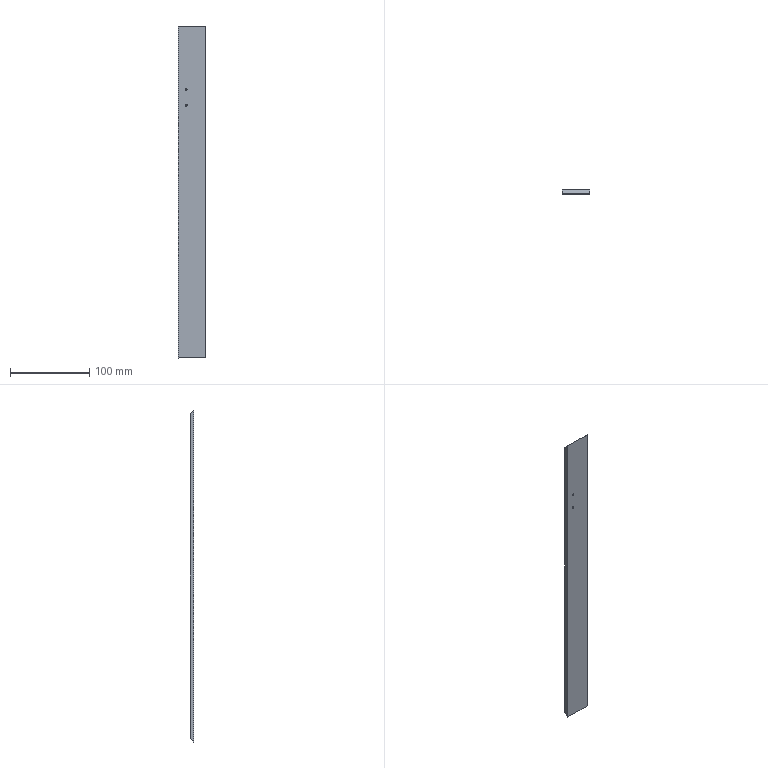Part | STEP file | 09-25 Cover side plate 1 | 1 solid | 10 faces | box 35 x 5 x 420 mm | volume 72576 mm3 | plane 6 | cylinder 4 | commonest cylinder face diameters 2.5 x4
STEP:
#1=CARTESIAN_POINT('',(0.,0.,0.));
#2=DIRECTION('',(0.,0.,1.));
#3=DIRECTION('',(1.,0.,0.));
#4=AXIS2_PLACEMENT_3D('',#1,#2,#3);
#5=CARTESIAN_POINT('',(11.25,5.,-80.));
#6=VERTEX_POINT('',#5);
#7=CARTESIAN_POINT('',(11.25,0.,-80.));
#8=VERTEX_POINT('',#7);
#9=CARTESIAN_POINT('',(11.25,5.,-80.));
#10=DIRECTION('',(0.,-1.,0.));
#11=VECTOR('',#10,1.);
#12=LINE('',#9,#11);
#13=CARTESIAN_POINT('',(10.,5.,-80.));
#14=DIRECTION('',(0.,-1.,0.));
#15=DIRECTION('',(1.,0.,0.));
#16=AXIS2_PLACEMENT_3D('',#13,#14,#15);
#17=CYLINDRICAL_SURFACE('',#16,1.25);
#18=CARTESIAN_POINT('',(6.283,0.));
#19=DIRECTION('',(0.,1.));
#20=VECTOR('',#19,1.);
#21=LINE('',#18,#20);
#22=(GEOMETRIC_REPRESENTATION_CONTEXT(2)PARAMETRIC_REPRESENTATION_CONTEXT()REPRESENTATION_CONTEXT('',''));
#23=DEFINITIONAL_REPRESENTATION('',(#21),#22);
#24=PCURVE('',#17,#23);
#25=CARTESIAN_POINT('',(10.,5.,-80.));
#26=DIRECTION('',(0.,-1.,0.));
#27=DIRECTION('',(1.,0.,0.));
#28=AXIS2_PLACEMENT_3D('',#25,#26,#27);
#29=CYLINDRICAL_SURFACE('',#28,1.25);
#30=CARTESIAN_POINT('',(0.,0.));
#31=DIRECTION('',(0.,1.));
#32=VECTOR('',#31,1.);
#33=LINE('',#30,#32);
#34=(GEOMETRIC_REPRESENTATION_CONTEXT(2)PARAMETRIC_REPRESENTATION_CONTEXT()REPRESENTATION_CONTEXT('',''));
#35=DEFINITIONAL_REPRESENTATION('',(#33),#34);
#36=PCURVE('',#29,#35);
#37=SURFACE_CURVE('',#12,(#24,#36),.PCURVE_S1.);
#38=EDGE_CURVE('',#6,#8,#37,.T.);
#39=ORIENTED_EDGE('',*,*,#38,.T.);
#40=CARTESIAN_POINT('',(8.75,0.,-80.));
#41=VERTEX_POINT('',#40);
#42=CARTESIAN_POINT('',(10.,0.,-80.));
#43=DIRECTION('',(0.,-1.,0.));
#44=DIRECTION('',(1.,0.,0.));
#45=AXIS2_PLACEMENT_3D('',#42,#43,#44);
#46=CIRCLE('',#45,1.25);
#47=CARTESIAN_POINT('',(0.,5.));
#48=DIRECTION('',(1.,0.));
#49=VECTOR('',#48,1.);
#50=LINE('',#47,#49);
#51=(GEOMETRIC_REPRESENTATION_CONTEXT(2)PARAMETRIC_REPRESENTATION_CONTEXT()REPRESENTATION_CONTEXT('',''));
#52=DEFINITIONAL_REPRESENTATION('',(#50),#51);
#53=PCURVE('',#17,#52);
#54=CARTESIAN_POINT('',(0.,0.,-420.));
#55=DIRECTION('',(0.,1.,0.));
#56=DIRECTION('',(0.,0.,1.));
#57=AXIS2_PLACEMENT_3D('',#54,#55,#56);
#58=PLANE('',#57);
#59=CARTESIAN_POINT('',(340.,11.25));
#60=CARTESIAN_POINT('',(342.165,11.25));
#61=CARTESIAN_POINT('',(341.083,9.375));
#62=CARTESIAN_POINT('',(340.,7.5));
#63=CARTESIAN_POINT('',(338.917,9.375));
#64=CARTESIAN_POINT('',(337.835,11.25));
#65=CARTESIAN_POINT('',(340.,11.25));
#66=(BOUNDED_CURVE()B_SPLINE_CURVE(2,(#59,#60,#61,#62,#63,#64,#65),.UNSPECIFIED.,.T.,.F.)B_SPLINE_CURVE_WITH_KNOTS((1,2,2,2,2,1),(-2.094,0.,2.094,4.189,6.283,8.378),.UNSPECIFIED.)CURVE()GEOMETRIC_REPRESENTATION_ITEM()RATIONAL_B_SPLINE_CURVE((1.,0.5,1.,0.5,1.,0.5,1.))REPRESENTATION_ITEM(''));
#67=(GEOMETRIC_REPRESENTATION_CONTEXT(2)PARAMETRIC_REPRESENTATION_CONTEXT()REPRESENTATION_CONTEXT('',''));
#68=DEFINITIONAL_REPRESENTATION('',(#66),#67);
#69=PCURVE('',#58,#68);
#70=SURFACE_CURVE('',#46,(#53,#69),.PCURVE_S1.);
#71=EDGE_CURVE('',#41,#8,#70,.T.);
#72=ORIENTED_EDGE('',*,*,#71,.F.);
#73=CARTESIAN_POINT('',(8.75,5.,-80.));
#74=VERTEX_POINT('',#73);
#75=CARTESIAN_POINT('',(8.75,5.,-80.));
#76=DIRECTION('',(0.,-1.,0.));
#77=VECTOR('',#76,1.);
#78=LINE('',#75,#77);
#79=CARTESIAN_POINT('',(3.142,0.));
#80=DIRECTION('',(0.,1.));
#81=VECTOR('',#80,1.);
#82=LINE('',#79,#81);
#83=(GEOMETRIC_REPRESENTATION_CONTEXT(2)PARAMETRIC_REPRESENTATION_CONTEXT()REPRESENTATION_CONTEXT('',''));
#84=DEFINITIONAL_REPRESENTATION('',(#82),#83);
#85=PCURVE('',#17,#84);
#86=CARTESIAN_POINT('',(3.142,0.));
#87=DIRECTION('',(0.,1.));
#88=VECTOR('',#87,1.);
#89=LINE('',#86,#88);
#90=(GEOMETRIC_REPRESENTATION_CONTEXT(2)PARAMETRIC_REPRESENTATION_CONTEXT()REPRESENTATION_CONTEXT('',''));
#91=DEFINITIONAL_REPRESENTATION('',(#89),#90);
#92=PCURVE('',#29,#91);
#93=SURFACE_CURVE('',#78,(#85,#92),.PCURVE_S1.);
#94=EDGE_CURVE('',#74,#41,#93,.T.);
#95=ORIENTED_EDGE('',*,*,#94,.F.);
#96=CARTESIAN_POINT('',(10.,5.,-80.));
#97=DIRECTION('',(0.,1.,0.));
#98=DIRECTION('',(1.,0.,0.));
#99=AXIS2_PLACEMENT_3D('',#96,#97,#98);
#100=CIRCLE('',#99,1.25);
#101=CARTESIAN_POINT('',(6.283,0.));
#102=DIRECTION('',(-1.,0.));
#103=VECTOR('',#102,1.);
#104=LINE('',#101,#103);
#105=(GEOMETRIC_REPRESENTATION_CONTEXT(2)PARAMETRIC_REPRESENTATION_CONTEXT()REPRESENTATION_CONTEXT('',''));
#106=DEFINITIONAL_REPRESENTATION('',(#104),#105);
#107=PCURVE('',#17,#106);
#108=CARTESIAN_POINT('',(0.,5.,-5.));
#109=DIRECTION('',(0.,-1.,0.));
#110=DIRECTION('',(0.,0.,-1.));
#111=AXIS2_PLACEMENT_3D('',#108,#109,#110);
#112=PLANE('',#111);
#113=CARTESIAN_POINT('',(75.,11.25));
#114=CARTESIAN_POINT('',(77.165,11.25));
#115=CARTESIAN_POINT('',(76.083,9.375));
#116=CARTESIAN_POINT('',(75.,7.5));
#117=CARTESIAN_POINT('',(73.917,9.375));
#118=CARTESIAN_POINT('',(72.835,11.25));
#119=CARTESIAN_POINT('',(75.,11.25));
#120=(BOUNDED_CURVE()B_SPLINE_CURVE(2,(#113,#114,#115,#116,#117,#118,#119),.UNSPECIFIED.,.T.,.F.)B_SPLINE_CURVE_WITH_KNOTS((1,2,2,2,2,1),(-2.094,0.,2.094,4.189,6.283,8.378),.UNSPECIFIED.)CURVE()GEOMETRIC_REPRESENTATION_ITEM()RATIONAL_B_SPLINE_CURVE((1.,0.5,1.,0.5,1.,0.5,1.))REPRESENTATION_ITEM(''));
#121=(GEOMETRIC_REPRESENTATION_CONTEXT(2)PARAMETRIC_REPRESENTATION_CONTEXT()REPRESENTATION_CONTEXT('',''));
#122=DEFINITIONAL_REPRESENTATION('',(#120),#121);
#123=PCURVE('',#112,#122);
#124=SURFACE_CURVE('',#100,(#107,#123),.PCURVE_S1.);
#125=EDGE_CURVE('',#6,#74,#124,.T.);
#126=ORIENTED_EDGE('',*,*,#125,.F.);
#127=EDGE_LOOP('',(#39,#72,#95,#126));
#128=FACE_BOUND('',#127,.F.);
#129=ADVANCED_FACE('',(#128),#17,.F.);
#130=CARTESIAN_POINT('',(11.25,5.,-100.));
#131=VERTEX_POINT('',#130);
#132=CARTESIAN_POINT('',(11.25,0.,-100.));
#133=VERTEX_POINT('',#132);
#134=CARTESIAN_POINT('',(11.25,5.,-100.));
#135=DIRECTION('',(0.,-1.,0.));
#136=VECTOR('',#135,1.);
#137=LINE('',#134,#136);
#138=CARTESIAN_POINT('',(10.,5.,-100.));
#139=DIRECTION('',(0.,-1.,0.));
#140=DIRECTION('',(1.,0.,0.));
#141=AXIS2_PLACEMENT_3D('',#138,#139,#140);
#142=CYLINDRICAL_SURFACE('',#141,1.25);
#143=CARTESIAN_POINT('',(6.283,0.));
#144=DIRECTION('',(0.,1.));
#145=VECTOR('',#144,1.);
#146=LINE('',#143,#145);
#147=(GEOMETRIC_REPRESENTATION_CONTEXT(2)PARAMETRIC_REPRESENTATION_CONTEXT()REPRESENTATION_CONTEXT('',''));
#148=DEFINITIONAL_REPRESENTATION('',(#146),#147);
#149=PCURVE('',#142,#148);
#150=CARTESIAN_POINT('',(10.,5.,-100.));
#151=DIRECTION('',(0.,-1.,0.));
#152=DIRECTION('',(1.,0.,0.));
#153=AXIS2_PLACEMENT_3D('',#150,#151,#152);
#154=CYLINDRICAL_SURFACE('',#153,1.25);
#155=CARTESIAN_POINT('',(0.,0.));
#156=DIRECTION('',(0.,1.));
#157=VECTOR('',#156,1.);
#158=LINE('',#155,#157);
#159=(GEOMETRIC_REPRESENTATION_CONTEXT(2)PARAMETRIC_REPRESENTATION_CONTEXT()REPRESENTATION_CONTEXT('',''));
#160=DEFINITIONAL_REPRESENTATION('',(#158),#159);
#161=PCURVE('',#154,#160);
#162=SURFACE_CURVE('',#137,(#149,#161),.PCURVE_S1.);
#163=EDGE_CURVE('',#131,#133,#162,.T.);
#164=ORIENTED_EDGE('',*,*,#163,.T.);
#165=CARTESIAN_POINT('',(8.75,0.,-100.));
#166=VERTEX_POINT('',#165);
#167=CARTESIAN_POINT('',(10.,0.,-100.));
#168=DIRECTION('',(0.,-1.,0.));
#169=DIRECTION('',(1.,0.,0.));
#170=AXIS2_PLACEMENT_3D('',#167,#168,#169);
#171=CIRCLE('',#170,1.25);
#172=CARTESIAN_POINT('',(0.,5.));
#173=DIRECTION('',(1.,0.));
#174=VECTOR('',#173,1.);
#175=LINE('',#172,#174);
#176=(GEOMETRIC_REPRESENTATION_CONTEXT(2)PARAMETRIC_REPRESENTATION_CONTEXT()REPRESENTATION_CONTEXT('',''));
#177=DEFINITIONAL_REPRESENTATION('',(#175),#176);
#178=PCURVE('',#142,#177);
#179=CARTESIAN_POINT('',(320.,11.25));
#180=CARTESIAN_POINT('',(322.165,11.25));
#181=CARTESIAN_POINT('',(321.083,9.375));
#182=CARTESIAN_POINT('',(320.,7.5));
#183=CARTESIAN_POINT('',(318.917,9.375));
#184=CARTESIAN_POINT('',(317.835,11.25));
#185=CARTESIAN_POINT('',(320.,11.25));
#186=(BOUNDED_CURVE()B_SPLINE_CURVE(2,(#179,#180,#181,#182,#183,#184,#185),.UNSPECIFIED.,.T.,.F.)B_SPLINE_CURVE_WITH_KNOTS((1,2,2,2,2,1),(-2.094,0.,2.094,4.189,6.283,8.378),.UNSPECIFIED.)CURVE()GEOMETRIC_REPRESENTATION_ITEM()RATIONAL_B_SPLINE_CURVE((1.,0.5,1.,0.5,1.,0.5,1.))REPRESENTATION_ITEM(''));
#187=(GEOMETRIC_REPRESENTATION_CONTEXT(2)PARAMETRIC_REPRESENTATION_CONTEXT()REPRESENTATION_CONTEXT('',''));
#188=DEFINITIONAL_REPRESENTATION('',(#186),#187);
#189=PCURVE('',#58,#188);
#190=SURFACE_CURVE('',#171,(#178,#189),.PCURVE_S1.);
#191=EDGE_CURVE('',#166,#133,#190,.T.);
#192=ORIENTED_EDGE('',*,*,#191,.F.);
#193=CARTESIAN_POINT('',(8.75,5.,-100.));
#194=VERTEX_POINT('',#193);
#195=CARTESIAN_POINT('',(8.75,5.,-100.));
#196=DIRECTION('',(0.,-1.,0.));
#197=VECTOR('',#196,1.);
#198=LINE('',#195,#197);
#199=CARTESIAN_POINT('',(3.142,0.));
#200=DIRECTION('',(0.,1.));
#201=VECTOR('',#200,1.);
#202=LINE('',#199,#201);
#203=(GEOMETRIC_REPRESENTATION_CONTEXT(2)PARAMETRIC_REPRESENTATION_CONTEXT()REPRESENTATION_CONTEXT('',''));
#204=DEFINITIONAL_REPRESENTATION('',(#202),#203);
#205=PCURVE('',#142,#204);
#206=CARTESIAN_POINT('',(3.142,0.));
#207=DIRECTION('',(0.,1.));
#208=VECTOR('',#207,1.);
#209=LINE('',#206,#208);
#210=(GEOMETRIC_REPRESENTATION_CONTEXT(2)PARAMETRIC_REPRESENTATION_CONTEXT()REPRESENTATION_CONTEXT('',''));
#211=DEFINITIONAL_REPRESENTATION('',(#209),#210);
#212=PCURVE('',#154,#211);
#213=SURFACE_CURVE('',#198,(#205,#212),.PCURVE_S1.);
#214=EDGE_CURVE('',#194,#166,#213,.T.);
#215=ORIENTED_EDGE('',*,*,#214,.F.);
#216=CARTESIAN_POINT('',(10.,5.,-100.));
#217=DIRECTION('',(0.,1.,0.));
#218=DIRECTION('',(1.,0.,0.));
#219=AXIS2_PLACEMENT_3D('',#216,#217,#218);
#220=CIRCLE('',#219,1.25);
#221=CARTESIAN_POINT('',(6.283,0.));
#222=DIRECTION('',(-1.,0.));
#223=VECTOR('',#222,1.);
#224=LINE('',#221,#223);
#225=(GEOMETRIC_REPRESENTATION_CONTEXT(2)PARAMETRIC_REPRESENTATION_CONTEXT()REPRESENTATION_CONTEXT('',''));
#226=DEFINITIONAL_REPRESENTATION('',(#224),#225);
#227=PCURVE('',#142,#226);
#228=CARTESIAN_POINT('',(95.,11.25));
#229=CARTESIAN_POINT('',(97.165,11.25));
#230=CARTESIAN_POINT('',(96.083,9.375));
#231=CARTESIAN_POINT('',(95.,7.5));
#232=CARTESIAN_POINT('',(93.917,9.375));
#233=CARTESIAN_POINT('',(92.835,11.25));
#234=CARTESIAN_POINT('',(95.,11.25));
#235=(BOUNDED_CURVE()B_SPLINE_CURVE(2,(#228,#229,#230,#231,#232,#233,#234),.UNSPECIFIED.,.T.,.F.)B_SPLINE_CURVE_WITH_KNOTS((1,2,2,2,2,1),(-2.094,0.,2.094,4.189,6.283,8.378),.UNSPECIFIED.)CURVE()GEOMETRIC_REPRESENTATION_ITEM()RATIONAL_B_SPLINE_CURVE((1.,0.5,1.,0.5,1.,0.5,1.))REPRESENTATION_ITEM(''));
#236=(GEOMETRIC_REPRESENTATION_CONTEXT(2)PARAMETRIC_REPRESENTATION_CONTEXT()REPRESENTATION_CONTEXT('',''));
#237=DEFINITIONAL_REPRESENTATION('',(#235),#236);
#238=PCURVE('',#112,#237);
#239=SURFACE_CURVE('',#220,(#227,#238),.PCURVE_S1.);
#240=EDGE_CURVE('',#131,#194,#239,.T.);
#241=ORIENTED_EDGE('',*,*,#240,.F.);
#242=EDGE_LOOP('',(#164,#192,#215,#241));
#243=FACE_BOUND('',#242,.F.);
#244=ADVANCED_FACE('',(#243),#142,.F.);
#245=CARTESIAN_POINT('',(10.,0.,-80.));
#246=DIRECTION('',(0.,-1.,0.));
#247=DIRECTION('',(1.,0.,0.));
#248=AXIS2_PLACEMENT_3D('',#245,#246,#247);
#249=CIRCLE('',#248,1.25);
#250=CARTESIAN_POINT('',(0.,5.));
#251=DIRECTION('',(1.,0.));
#252=VECTOR('',#251,1.);
#253=LINE('',#250,#252);
#254=(GEOMETRIC_REPRESENTATION_CONTEXT(2)PARAMETRIC_REPRESENTATION_CONTEXT()REPRESENTATION_CONTEXT('',''));
#255=DEFINITIONAL_REPRESENTATION('',(#253),#254);
#256=PCURVE('',#29,#255);
#257=CARTESIAN_POINT('',(340.,11.25));
#258=CARTESIAN_POINT('',(342.165,11.25));
#259=CARTESIAN_POINT('',(341.083,9.375));
#260=CARTESIAN_POINT('',(340.,7.5));
#261=CARTESIAN_POINT('',(338.917,9.375));
#262=CARTESIAN_POINT('',(337.835,11.25));
#263=CARTESIAN_POINT('',(340.,11.25));
#264=(BOUNDED_CURVE()B_SPLINE_CURVE(2,(#257,#258,#259,#260,#261,#262,#263),.UNSPECIFIED.,.T.,.F.)B_SPLINE_CURVE_WITH_KNOTS((1,2,2,2,2,1),(-2.094,0.,2.094,4.189,6.283,8.378),.UNSPECIFIED.)CURVE()GEOMETRIC_REPRESENTATION_ITEM()RATIONAL_B_SPLINE_CURVE((1.,0.5,1.,0.5,1.,0.5,1.))REPRESENTATION_ITEM(''));
#265=(GEOMETRIC_REPRESENTATION_CONTEXT(2)PARAMETRIC_REPRESENTATION_CONTEXT()REPRESENTATION_CONTEXT('',''));
#266=DEFINITIONAL_REPRESENTATION('',(#264),#265);
#267=PCURVE('',#58,#266);
#268=SURFACE_CURVE('',#249,(#256,#267),.PCURVE_S1.);
#269=EDGE_CURVE('',#8,#41,#268,.T.);
#270=ORIENTED_EDGE('',*,*,#269,.F.);
#271=ORIENTED_EDGE('',*,*,#38,.F.);
#272=CARTESIAN_POINT('',(10.,5.,-80.));
#273=DIRECTION('',(0.,1.,0.));
#274=DIRECTION('',(1.,0.,0.));
#275=AXIS2_PLACEMENT_3D('',#272,#273,#274);
#276=CIRCLE('',#275,1.25);
#277=CARTESIAN_POINT('',(6.283,0.));
#278=DIRECTION('',(-1.,0.));
#279=VECTOR('',#278,1.);
#280=LINE('',#277,#279);
#281=(GEOMETRIC_REPRESENTATION_CONTEXT(2)PARAMETRIC_REPRESENTATION_CONTEXT()REPRESENTATION_CONTEXT('',''));
#282=DEFINITIONAL_REPRESENTATION('',(#280),#281);
#283=PCURVE('',#29,#282);
#284=CARTESIAN_POINT('',(75.,11.25));
#285=CARTESIAN_POINT('',(77.165,11.25));
#286=CARTESIAN_POINT('',(76.083,9.375));
#287=CARTESIAN_POINT('',(75.,7.5));
#288=CARTESIAN_POINT('',(73.917,9.375));
#289=CARTESIAN_POINT('',(72.835,11.25));
#290=CARTESIAN_POINT('',(75.,11.25));
#291=(BOUNDED_CURVE()B_SPLINE_CURVE(2,(#284,#285,#286,#287,#288,#289,#290),.UNSPECIFIED.,.T.,.F.)B_SPLINE_CURVE_WITH_KNOTS((1,2,2,2,2,1),(-2.094,0.,2.094,4.189,6.283,8.378),.UNSPECIFIED.)CURVE()GEOMETRIC_REPRESENTATION_ITEM()RATIONAL_B_SPLINE_CURVE((1.,0.5,1.,0.5,1.,0.5,1.))REPRESENTATION_ITEM(''));
#292=(GEOMETRIC_REPRESENTATION_CONTEXT(2)PARAMETRIC_REPRESENTATION_CONTEXT()REPRESENTATION_CONTEXT('',''));
#293=DEFINITIONAL_REPRESENTATION('',(#291),#292);
#294=PCURVE('',#112,#293);
#295=SURFACE_CURVE('',#276,(#283,#294),.PCURVE_S1.);
#296=EDGE_CURVE('',#74,#6,#295,.T.);
#297=ORIENTED_EDGE('',*,*,#296,.F.);
#298=ORIENTED_EDGE('',*,*,#94,.T.);
#299=EDGE_LOOP('',(#270,#271,#297,#298));
#300=FACE_BOUND('',#299,.F.);
#301=ADVANCED_FACE('',(#300),#29,.F.);
#302=CARTESIAN_POINT('',(10.,0.,-100.));
#303=DIRECTION('',(0.,-1.,0.));
#304=DIRECTION('',(1.,0.,0.));
#305=AXIS2_PLACEMENT_3D('',#302,#303,#304);
#306=CIRCLE('',#305,1.25);
#307=CARTESIAN_POINT('',(320.,11.25));
#308=CARTESIAN_POINT('',(322.165,11.25));
#309=CARTESIAN_POINT('',(321.083,9.375));
#310=CARTESIAN_POINT('',(320.,7.5));
#311=CARTESIAN_POINT('',(318.917,9.375));
#312=CARTESIAN_POINT('',(317.835,11.25));
#313=CARTESIAN_POINT('',(320.,11.25));
#314=(BOUNDED_CURVE()B_SPLINE_CURVE(2,(#307,#308,#309,#310,#311,#312,#313),.UNSPECIFIED.,.T.,.F.)B_SPLINE_CURVE_WITH_KNOTS((1,2,2,2,2,1),(-2.094,0.,2.094,4.189,6.283,8.378),.UNSPECIFIED.)CURVE()GEOMETRIC_REPRESENTATION_ITEM()RATIONAL_B_SPLINE_CURVE((1.,0.5,1.,0.5,1.,0.5,1.))REPRESENTATION_ITEM(''));
#315=(GEOMETRIC_REPRESENTATION_CONTEXT(2)PARAMETRIC_REPRESENTATION_CONTEXT()REPRESENTATION_CONTEXT('',''));
#316=DEFINITIONAL_REPRESENTATION('',(#314),#315);
#317=PCURVE('',#58,#316);
#318=CARTESIAN_POINT('',(0.,5.));
#319=DIRECTION('',(1.,0.));
#320=VECTOR('',#319,1.);
#321=LINE('',#318,#320);
#322=(GEOMETRIC_REPRESENTATION_CONTEXT(2)PARAMETRIC_REPRESENTATION_CONTEXT()REPRESENTATION_CONTEXT('',''));
#323=DEFINITIONAL_REPRESENTATION('',(#321),#322);
#324=PCURVE('',#154,#323);
#325=SURFACE_CURVE('',#306,(#317,#324),.PCURVE_S1.);
#326=EDGE_CURVE('',#133,#166,#325,.T.);
#327=ORIENTED_EDGE('',*,*,#326,.F.);
#328=ORIENTED_EDGE('',*,*,#191,.F.);
#329=EDGE_LOOP('',(#327,#328));
#330=FACE_BOUND('',#329,.T.);
#331=ORIENTED_EDGE('',*,*,#269,.F.);
#332=ORIENTED_EDGE('',*,*,#71,.F.);
#333=EDGE_LOOP('',(#331,#332));
#334=FACE_BOUND('',#333,.T.);
#335=CARTESIAN_POINT('',(35.,0.,-420.));
#336=VERTEX_POINT('',#335);
#337=CARTESIAN_POINT('',(0.,0.,-420.));
#338=VERTEX_POINT('',#337);
#339=CARTESIAN_POINT('',(17.5,0.,-420.));
#340=DIRECTION('',(-1.,0.,0.));
#341=VECTOR('',#340,1.);
#342=LINE('',#339,#341);
#343=CARTESIAN_POINT('',(0.,17.5));
#344=DIRECTION('',(0.,-1.));
#345=VECTOR('',#344,1.);
#346=LINE('',#343,#345);
#347=(GEOMETRIC_REPRESENTATION_CONTEXT(2)PARAMETRIC_REPRESENTATION_CONTEXT()REPRESENTATION_CONTEXT('',''));
#348=DEFINITIONAL_REPRESENTATION('',(#346),#347);
#349=PCURVE('',#58,#348);
#350=CARTESIAN_POINT('',(0.,5.,-415.));
#351=DIRECTION('',(0.,-0.7071,0.7071));
#352=DIRECTION('',(0.,-0.7071,-0.7071));
#353=AXIS2_PLACEMENT_3D('',#350,#351,#352);
#354=PLANE('',#353);
#355=CARTESIAN_POINT('',(7.071,17.5));
#356=DIRECTION('',(0.,-1.));
#357=VECTOR('',#356,1.);
#358=LINE('',#355,#357);
#359=(GEOMETRIC_REPRESENTATION_CONTEXT(2)PARAMETRIC_REPRESENTATION_CONTEXT()REPRESENTATION_CONTEXT('',''));
#360=DEFINITIONAL_REPRESENTATION('',(#358),#359);
#361=PCURVE('',#354,#360);
#362=SURFACE_CURVE('',#342,(#349,#361),.PCURVE_S1.);
#363=EDGE_CURVE('',#336,#338,#362,.T.);
#364=ORIENTED_EDGE('',*,*,#363,.F.);
#365=CARTESIAN_POINT('',(35.,0.,-0.000000052));
#366=VERTEX_POINT('',#365);
#367=CARTESIAN_POINT('',(35.,0.,-210.));
#368=DIRECTION('',(0.,0.,-1.));
#369=VECTOR('',#368,1.);
#370=LINE('',#367,#369);
#371=CARTESIAN_POINT('',(210.,35.));
#372=DIRECTION('',(-1.,0.));
#373=VECTOR('',#372,1.);
#374=LINE('',#371,#373);
#375=(GEOMETRIC_REPRESENTATION_CONTEXT(2)PARAMETRIC_REPRESENTATION_CONTEXT()REPRESENTATION_CONTEXT('',''));
#376=DEFINITIONAL_REPRESENTATION('',(#374),#375);
#377=PCURVE('',#58,#376);
#378=CARTESIAN_POINT('',(35.,0.,2.52));
#379=DIRECTION('',(1.,0.,0.));
#380=DIRECTION('',(0.,0.,-1.));
#381=AXIS2_PLACEMENT_3D('',#378,#379,#380);
#382=PLANE('',#381);
#383=CARTESIAN_POINT('',(212.52,0.));
#384=DIRECTION('',(1.,0.));
#385=VECTOR('',#384,1.);
#386=LINE('',#383,#385);
#387=(GEOMETRIC_REPRESENTATION_CONTEXT(2)PARAMETRIC_REPRESENTATION_CONTEXT()REPRESENTATION_CONTEXT('',''));
#388=DEFINITIONAL_REPRESENTATION('',(#386),#387);
#389=PCURVE('',#382,#388);
#390=SURFACE_CURVE('',#370,(#377,#389),.PCURVE_S1.);
#391=EDGE_CURVE('',#366,#336,#390,.T.);
#392=ORIENTED_EDGE('',*,*,#391,.F.);
#393=CARTESIAN_POINT('',(0.,0.,0.));
#394=VERTEX_POINT('',#393);
#395=CARTESIAN_POINT('',(17.5,0.,0.));
#396=DIRECTION('',(1.,0.,0.));
#397=VECTOR('',#396,1.);
#398=LINE('',#395,#397);
#399=CARTESIAN_POINT('',(420.,17.5));
#400=DIRECTION('',(0.,1.));
#401=VECTOR('',#400,1.);
#402=LINE('',#399,#401);
#403=(GEOMETRIC_REPRESENTATION_CONTEXT(2)PARAMETRIC_REPRESENTATION_CONTEXT()REPRESENTATION_CONTEXT('',''));
#404=DEFINITIONAL_REPRESENTATION('',(#402),#403);
#405=PCURVE('',#58,#404);
#406=CARTESIAN_POINT('',(0.,0.,0.));
#407=DIRECTION('',(0.,-0.7071,-0.7071));
#408=DIRECTION('',(0.,0.7071,-0.7071));
#409=AXIS2_PLACEMENT_3D('',#406,#407,#408);
#410=PLANE('',#409);
#411=CARTESIAN_POINT('',(0.,17.5));
#412=DIRECTION('',(0.,1.));
#413=VECTOR('',#412,1.);
#414=LINE('',#411,#413);
#415=(GEOMETRIC_REPRESENTATION_CONTEXT(2)PARAMETRIC_REPRESENTATION_CONTEXT()REPRESENTATION_CONTEXT('',''));
#416=DEFINITIONAL_REPRESENTATION('',(#414),#415);
#417=PCURVE('',#410,#416);
#418=SURFACE_CURVE('',#398,(#405,#417),.PCURVE_S1.);
#419=EDGE_CURVE('',#394,#366,#418,.T.);
#420=ORIENTED_EDGE('',*,*,#419,.F.);
#421=CARTESIAN_POINT('',(0.,0.,-210.));
#422=DIRECTION('',(0.,0.,1.));
#423=VECTOR('',#422,1.);
#424=LINE('',#421,#423);
#425=CARTESIAN_POINT('',(210.,0.));
#426=DIRECTION('',(1.,0.));
#427=VECTOR('',#426,1.);
#428=LINE('',#425,#427);
#429=(GEOMETRIC_REPRESENTATION_CONTEXT(2)PARAMETRIC_REPRESENTATION_CONTEXT()REPRESENTATION_CONTEXT('',''));
#430=DEFINITIONAL_REPRESENTATION('',(#428),#429);
#431=PCURVE('',#58,#430);
#432=CARTESIAN_POINT('',(0.,0.,2.52));
#433=DIRECTION('',(1.,0.,0.));
#434=DIRECTION('',(0.,0.,-1.));
#435=AXIS2_PLACEMENT_3D('',#432,#433,#434);
#436=PLANE('',#435);
#437=CARTESIAN_POINT('',(212.52,0.));
#438=DIRECTION('',(-1.,0.));
#439=VECTOR('',#438,1.);
#440=LINE('',#437,#439);
#441=(GEOMETRIC_REPRESENTATION_CONTEXT(2)PARAMETRIC_REPRESENTATION_CONTEXT()REPRESENTATION_CONTEXT('',''));
#442=DEFINITIONAL_REPRESENTATION('',(#440),#441);
#443=PCURVE('',#436,#442);
#444=SURFACE_CURVE('',#424,(#431,#443),.PCURVE_S1.);
#445=EDGE_CURVE('',#338,#394,#444,.T.);
#446=ORIENTED_EDGE('',*,*,#445,.F.);
#447=EDGE_LOOP('',(#364,#392,#420,#446));
#448=FACE_BOUND('',#447,.T.);
#449=ADVANCED_FACE('',(#330,#334,#448),#58,.F.);
#450=ORIENTED_EDGE('',*,*,#240,.F.);
#451=CARTESIAN_POINT('',(10.,5.,-100.));
#452=DIRECTION('',(0.,1.,0.));
#453=DIRECTION('',(1.,0.,0.));
#454=AXIS2_PLACEMENT_3D('',#451,#452,#453);
#455=CIRCLE('',#454,1.25);
#456=CARTESIAN_POINT('',(95.,11.25));
#457=CARTESIAN_POINT('',(97.165,11.25));
#458=CARTESIAN_POINT('',(96.083,9.375));
#459=CARTESIAN_POINT('',(95.,7.5));
#460=CARTESIAN_POINT('',(93.917,9.375));
#461=CARTESIAN_POINT('',(92.835,11.25));
#462=CARTESIAN_POINT('',(95.,11.25));
#463=(BOUNDED_CURVE()B_SPLINE_CURVE(2,(#456,#457,#458,#459,#460,#461,#462),.UNSPECIFIED.,.T.,.F.)B_SPLINE_CURVE_WITH_KNOTS((1,2,2,2,2,1),(-2.094,0.,2.094,4.189,6.283,8.378),.UNSPECIFIED.)CURVE()GEOMETRIC_REPRESENTATION_ITEM()RATIONAL_B_SPLINE_CURVE((1.,0.5,1.,0.5,1.,0.5,1.))REPRESENTATION_ITEM(''));
#464=(GEOMETRIC_REPRESENTATION_CONTEXT(2)PARAMETRIC_REPRESENTATION_CONTEXT()REPRESENTATION_CONTEXT('',''));
#465=DEFINITIONAL_REPRESENTATION('',(#463),#464);
#466=PCURVE('',#112,#465);
#467=CARTESIAN_POINT('',(6.283,0.));
#468=DIRECTION('',(-1.,0.));
#469=VECTOR('',#468,1.);
#470=LINE('',#467,#469);
#471=(GEOMETRIC_REPRESENTATION_CONTEXT(2)PARAMETRIC_REPRESENTATION_CONTEXT()REPRESENTATION_CONTEXT('',''));
#472=DEFINITIONAL_REPRESENTATION('',(#470),#471);
#473=PCURVE('',#154,#472);
#474=SURFACE_CURVE('',#455,(#466,#473),.PCURVE_S1.);
#475=EDGE_CURVE('',#194,#131,#474,.T.);
#476=ORIENTED_EDGE('',*,*,#475,.F.);
#477=EDGE_LOOP('',(#450,#476));
#478=FACE_BOUND('',#477,.T.);
#479=ORIENTED_EDGE('',*,*,#125,.F.);
#480=ORIENTED_EDGE('',*,*,#296,.F.);
#481=EDGE_LOOP('',(#479,#480));
#482=FACE_BOUND('',#481,.T.);
#483=CARTESIAN_POINT('',(35.,5.,-5.));
#484=VERTEX_POINT('',#483);
#485=CARTESIAN_POINT('',(0.,5.,-5.));
#486=VERTEX_POINT('',#485);
#487=CARTESIAN_POINT('',(17.5,5.,-5.));
#488=DIRECTION('',(-1.,0.,0.));
#489=VECTOR('',#488,1.);
#490=LINE('',#487,#489);
#491=CARTESIAN_POINT('',(0.,17.5));
#492=DIRECTION('',(0.,-1.));
#493=VECTOR('',#492,1.);
#494=LINE('',#491,#493);
#495=(GEOMETRIC_REPRESENTATION_CONTEXT(2)PARAMETRIC_REPRESENTATION_CONTEXT()REPRESENTATION_CONTEXT('',''));
#496=DEFINITIONAL_REPRESENTATION('',(#494),#495);
#497=PCURVE('',#112,#496);
#498=CARTESIAN_POINT('',(7.071,17.5));
#499=DIRECTION('',(0.,-1.));
#500=VECTOR('',#499,1.);
#501=LINE('',#498,#500);
#502=(GEOMETRIC_REPRESENTATION_CONTEXT(2)PARAMETRIC_REPRESENTATION_CONTEXT()REPRESENTATION_CONTEXT('',''));
#503=DEFINITIONAL_REPRESENTATION('',(#501),#502);
#504=PCURVE('',#410,#503);
#505=SURFACE_CURVE('',#490,(#497,#504),.PCURVE_S1.);
#506=EDGE_CURVE('',#484,#486,#505,.T.);
#507=ORIENTED_EDGE('',*,*,#506,.F.);
#508=CARTESIAN_POINT('',(35.,5.,-415.));
#509=VERTEX_POINT('',#508);
#510=CARTESIAN_POINT('',(35.,5.,-210.));
#511=DIRECTION('',(0.,0.,1.));
#512=VECTOR('',#511,1.);
#513=LINE('',#510,#512);
#514=CARTESIAN_POINT('',(205.,35.));
#515=DIRECTION('',(-1.,0.));
#516=VECTOR('',#515,1.);
#517=LINE('',#514,#516);
#518=(GEOMETRIC_REPRESENTATION_CONTEXT(2)PARAMETRIC_REPRESENTATION_CONTEXT()REPRESENTATION_CONTEXT('',''));
#519=DEFINITIONAL_REPRESENTATION('',(#517),#518);
#520=PCURVE('',#112,#519);
#521=CARTESIAN_POINT('',(212.52,5.));
#522=DIRECTION('',(-1.,0.));
#523=VECTOR('',#522,1.);
#524=LINE('',#521,#523);
#525=(GEOMETRIC_REPRESENTATION_CONTEXT(2)PARAMETRIC_REPRESENTATION_CONTEXT()REPRESENTATION_CONTEXT('',''));
#526=DEFINITIONAL_REPRESENTATION('',(#524),#525);
#527=PCURVE('',#382,#526);
#528=SURFACE_CURVE('',#513,(#520,#527),.PCURVE_S1.);
#529=EDGE_CURVE('',#509,#484,#528,.T.);
#530=ORIENTED_EDGE('',*,*,#529,.F.);
#531=CARTESIAN_POINT('',(0.,5.,-415.));
#532=VERTEX_POINT('',#531);
#533=CARTESIAN_POINT('',(17.5,5.,-415.));
#534=DIRECTION('',(1.,0.,0.));
#535=VECTOR('',#534,1.);
#536=LINE('',#533,#535);
#537=CARTESIAN_POINT('',(410.,17.5));
#538=DIRECTION('',(0.,1.));
#539=VECTOR('',#538,1.);
#540=LINE('',#537,#539);
#541=(GEOMETRIC_REPRESENTATION_CONTEXT(2)PARAMETRIC_REPRESENTATION_CONTEXT()REPRESENTATION_CONTEXT('',''));
#542=DEFINITIONAL_REPRESENTATION('',(#540),#541);
#543=PCURVE('',#112,#542);
#544=CARTESIAN_POINT('',(0.,17.5));
#545=DIRECTION('',(0.,1.));
#546=VECTOR('',#545,1.);
#547=LINE('',#544,#546);
#548=(GEOMETRIC_REPRESENTATION_CONTEXT(2)PARAMETRIC_REPRESENTATION_CONTEXT()REPRESENTATION_CONTEXT('',''));
#549=DEFINITIONAL_REPRESENTATION('',(#547),#548);
#550=PCURVE('',#354,#549);
#551=SURFACE_CURVE('',#536,(#543,#550),.PCURVE_S1.);
#552=EDGE_CURVE('',#532,#509,#551,.T.);
#553=ORIENTED_EDGE('',*,*,#552,.F.);
#554=CARTESIAN_POINT('',(0.,5.,-210.));
#555=DIRECTION('',(0.,0.,-1.));
#556=VECTOR('',#555,1.);
#557=LINE('',#554,#556);
#558=CARTESIAN_POINT('',(205.,0.));
#559=DIRECTION('',(1.,0.));
#560=VECTOR('',#559,1.);
#561=LINE('',#558,#560);
#562=(GEOMETRIC_REPRESENTATION_CONTEXT(2)PARAMETRIC_REPRESENTATION_CONTEXT()REPRESENTATION_CONTEXT('',''));
#563=DEFINITIONAL_REPRESENTATION('',(#561),#562);
#564=PCURVE('',#112,#563);
#565=CARTESIAN_POINT('',(212.52,5.));
#566=DIRECTION('',(1.,0.));
#567=VECTOR('',#566,1.);
#568=LINE('',#565,#567);
#569=(GEOMETRIC_REPRESENTATION_CONTEXT(2)PARAMETRIC_REPRESENTATION_CONTEXT()REPRESENTATION_CONTEXT('',''));
#570=DEFINITIONAL_REPRESENTATION('',(#568),#569);
#571=PCURVE('',#436,#570);
#572=SURFACE_CURVE('',#557,(#564,#571),.PCURVE_S1.);
#573=EDGE_CURVE('',#486,#532,#572,.T.);
#574=ORIENTED_EDGE('',*,*,#573,.F.);
#575=EDGE_LOOP('',(#507,#530,#553,#574));
#576=FACE_BOUND('',#575,.T.);
#577=ADVANCED_FACE('',(#478,#482,#576),#112,.F.);
#578=ORIENTED_EDGE('',*,*,#326,.F.);
#579=ORIENTED_EDGE('',*,*,#163,.F.);
#580=ORIENTED_EDGE('',*,*,#475,.F.);
#581=ORIENTED_EDGE('',*,*,#214,.T.);
#582=EDGE_LOOP('',(#578,#579,#580,#581));
#583=FACE_BOUND('',#582,.F.);
#584=ADVANCED_FACE('',(#583),#154,.F.);
#585=CARTESIAN_POINT('',(0.,0.,0.));
#586=DIRECTION('',(0.,-0.7071,0.7071));
#587=VECTOR('',#586,1.);
#588=LINE('',#585,#587);
#589=CARTESIAN_POINT('',(2.52,0.));
#590=DIRECTION('',(-0.7071,-0.7071));
#591=VECTOR('',#590,1.);
#592=LINE('',#589,#591);
#593=(GEOMETRIC_REPRESENTATION_CONTEXT(2)PARAMETRIC_REPRESENTATION_CONTEXT()REPRESENTATION_CONTEXT('',''));
#594=DEFINITIONAL_REPRESENTATION('',(#592),#593);
#595=PCURVE('',#436,#594);
#596=CARTESIAN_POINT('',(0.,0.));
#597=DIRECTION('',(-1.,0.));
#598=VECTOR('',#597,1.);
#599=LINE('',#596,#598);
#600=(GEOMETRIC_REPRESENTATION_CONTEXT(2)PARAMETRIC_REPRESENTATION_CONTEXT()REPRESENTATION_CONTEXT('',''));
#601=DEFINITIONAL_REPRESENTATION('',(#599),#600);
#602=PCURVE('',#410,#601);
#603=SURFACE_CURVE('',#588,(#595,#602),.PCURVE_S1.);
#604=EDGE_CURVE('',#486,#394,#603,.T.);
#605=ORIENTED_EDGE('',*,*,#604,.F.);
#606=ORIENTED_EDGE('',*,*,#573,.T.);
#607=CARTESIAN_POINT('',(0.,5.,-415.));
#608=DIRECTION('',(0.,0.7071,0.7071));
#609=VECTOR('',#608,1.);
#610=LINE('',#607,#609);
#611=CARTESIAN_POINT('',(417.52,5.));
#612=DIRECTION('',(-0.7071,0.7071));
#613=VECTOR('',#612,1.);
#614=LINE('',#611,#613);
#615=(GEOMETRIC_REPRESENTATION_CONTEXT(2)PARAMETRIC_REPRESENTATION_CONTEXT()REPRESENTATION_CONTEXT('',''));
#616=DEFINITIONAL_REPRESENTATION('',(#614),#615);
#617=PCURVE('',#436,#616);
#618=CARTESIAN_POINT('',(0.,0.));
#619=DIRECTION('',(-1.,0.));
#620=VECTOR('',#619,1.);
#621=LINE('',#618,#620);
#622=(GEOMETRIC_REPRESENTATION_CONTEXT(2)PARAMETRIC_REPRESENTATION_CONTEXT()REPRESENTATION_CONTEXT('',''));
#623=DEFINITIONAL_REPRESENTATION('',(#621),#622);
#624=PCURVE('',#354,#623);
#625=SURFACE_CURVE('',#610,(#617,#624),.PCURVE_S1.);
#626=EDGE_CURVE('',#338,#532,#625,.T.);
#627=ORIENTED_EDGE('',*,*,#626,.F.);
#628=ORIENTED_EDGE('',*,*,#445,.T.);
#629=EDGE_LOOP('',(#605,#606,#627,#628));
#630=FACE_BOUND('',#629,.T.);
#631=ADVANCED_FACE('',(#630),#436,.F.);
#632=ORIENTED_EDGE('',*,*,#552,.T.);
#633=CARTESIAN_POINT('',(35.,2.5,-417.5));
#634=DIRECTION('',(0.,0.7071,0.7071));
#635=VECTOR('',#634,1.);
#636=LINE('',#633,#635);
#637=CARTESIAN_POINT('',(3.536,35.));
#638=DIRECTION('',(-1.,0.));
#639=VECTOR('',#638,1.);
#640=LINE('',#637,#639);
#641=(GEOMETRIC_REPRESENTATION_CONTEXT(2)PARAMETRIC_REPRESENTATION_CONTEXT()REPRESENTATION_CONTEXT('',''));
#642=DEFINITIONAL_REPRESENTATION('',(#640),#641);
#643=PCURVE('',#354,#642);
#644=CARTESIAN_POINT('',(420.02,2.5));
#645=DIRECTION('',(-0.7071,0.7071));
#646=VECTOR('',#645,1.);
#647=LINE('',#644,#646);
#648=(GEOMETRIC_REPRESENTATION_CONTEXT(2)PARAMETRIC_REPRESENTATION_CONTEXT()REPRESENTATION_CONTEXT('',''));
#649=DEFINITIONAL_REPRESENTATION('',(#647),#648);
#650=PCURVE('',#382,#649);
#651=SURFACE_CURVE('',#636,(#643,#650),.PCURVE_S1.);
#652=EDGE_CURVE('',#336,#509,#651,.T.);
#653=ORIENTED_EDGE('',*,*,#652,.F.);
#654=ORIENTED_EDGE('',*,*,#363,.T.);
#655=ORIENTED_EDGE('',*,*,#626,.T.);
#656=EDGE_LOOP('',(#632,#653,#654,#655));
#657=FACE_BOUND('',#656,.T.);
#658=ADVANCED_FACE('',(#657),#354,.F.);
#659=ORIENTED_EDGE('',*,*,#529,.T.);
#660=CARTESIAN_POINT('',(35.,5.,-5.));
#661=DIRECTION('',(0.,-0.7071,0.7071));
#662=VECTOR('',#661,1.);
#663=LINE('',#660,#662);
#664=CARTESIAN_POINT('',(7.52,5.));
#665=DIRECTION('',(-0.7071,-0.7071));
#666=VECTOR('',#665,1.);
#667=LINE('',#664,#666);
#668=(GEOMETRIC_REPRESENTATION_CONTEXT(2)PARAMETRIC_REPRESENTATION_CONTEXT()REPRESENTATION_CONTEXT('',''));
#669=DEFINITIONAL_REPRESENTATION('',(#667),#668);
#670=PCURVE('',#382,#669);
#671=CARTESIAN_POINT('',(7.071,35.));
#672=DIRECTION('',(-1.,0.));
#673=VECTOR('',#672,1.);
#674=LINE('',#671,#673);
#675=(GEOMETRIC_REPRESENTATION_CONTEXT(2)PARAMETRIC_REPRESENTATION_CONTEXT()REPRESENTATION_CONTEXT('',''));
#676=DEFINITIONAL_REPRESENTATION('',(#674),#675);
#677=PCURVE('',#410,#676);
#678=SURFACE_CURVE('',#663,(#670,#677),.PCURVE_S1.);
#679=EDGE_CURVE('',#484,#366,#678,.T.);
#680=ORIENTED_EDGE('',*,*,#679,.T.);
#681=ORIENTED_EDGE('',*,*,#391,.T.);
#682=ORIENTED_EDGE('',*,*,#652,.T.);
#683=EDGE_LOOP('',(#659,#680,#681,#682));
#684=FACE_BOUND('',#683,.T.);
#685=ADVANCED_FACE('',(#684),#382,.T.);
#686=ORIENTED_EDGE('',*,*,#419,.T.);
#687=ORIENTED_EDGE('',*,*,#679,.F.);
#688=ORIENTED_EDGE('',*,*,#506,.T.);
#689=ORIENTED_EDGE('',*,*,#604,.T.);
#690=EDGE_LOOP('',(#686,#687,#688,#689));
#691=FACE_BOUND('',#690,.T.);
#692=ADVANCED_FACE('',(#691),#410,.F.);
#693=CLOSED_SHELL('',(#129,#244,#301,#449,#577,#584,#631,#658,#685,#692));
#694=MANIFOLD_SOLID_BREP('',#693);
#695=(LENGTH_UNIT()NAMED_UNIT(*)SI_UNIT(.MILLI.,.METRE.));
#696=UNCERTAINTY_MEASURE_WITH_UNIT(LENGTH_MEASURE(0.0000001),#695,'','');
#697=(NAMED_UNIT(*)PLANE_ANGLE_UNIT()SI_UNIT($,.RADIAN.));
#698=(NAMED_UNIT(*)SI_UNIT($,.STERADIAN.)SOLID_ANGLE_UNIT());
#699=(GEOMETRIC_REPRESENTATION_CONTEXT(3)GLOBAL_UNCERTAINTY_ASSIGNED_CONTEXT((#696))GLOBAL_UNIT_ASSIGNED_CONTEXT((#695,#697,#698))REPRESENTATION_CONTEXT('',''));
#700=ADVANCED_BREP_SHAPE_REPRESENTATION('',(#4,#694),#699);